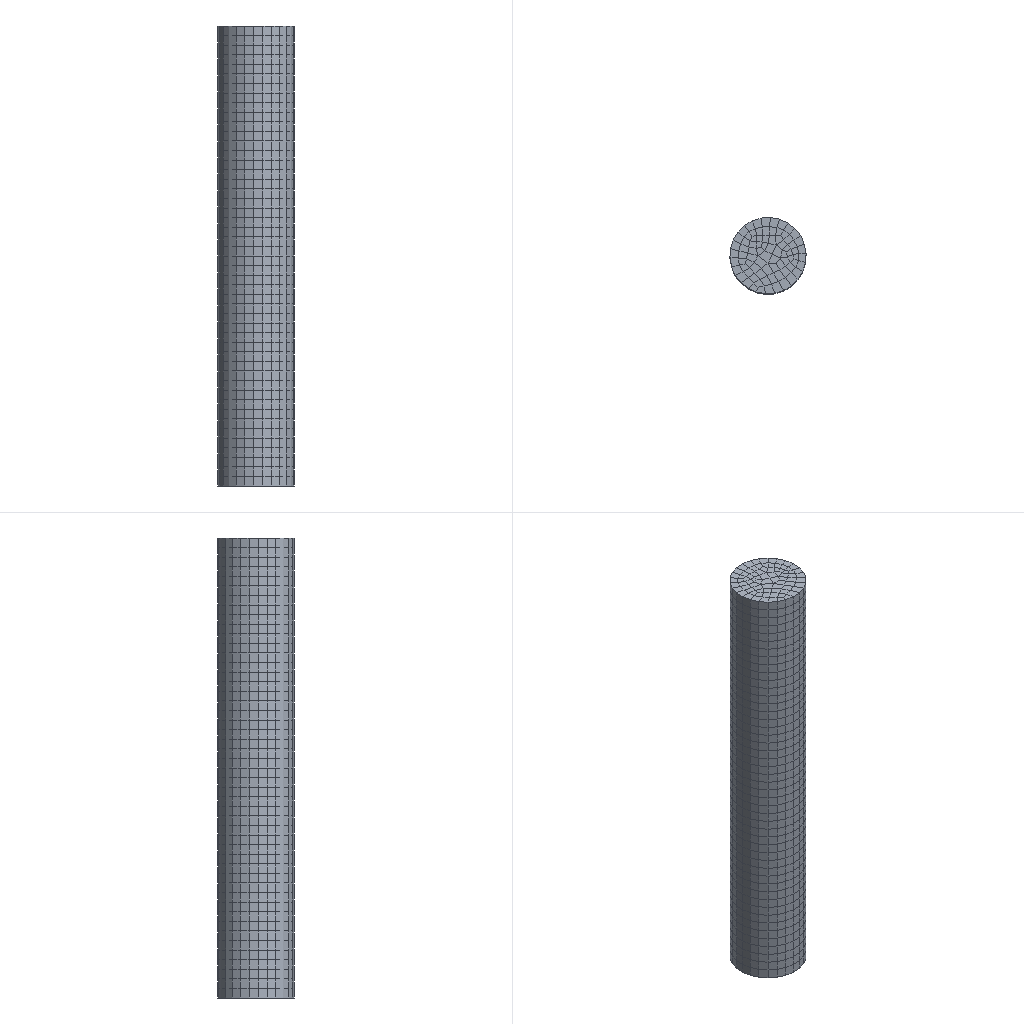Simulation study | abaqus
Set-up summary:
category,name,step,type,value,unit,region
solver,abaqus
solver,version,,,Abaqus/Explicit 2020
units,not stated in the deck,,not stated
analysis,deck,,transient,transient
load_step,Step-1,Step-1,transient
load_step,requested,,,1
mesh,nodes,,,17527
mesh,elements,,,16895
element_type,R3D3,,rigid,133
element_type,R3D4,,rigid,12970
element_type,C3D8R,,solid,3792
load,load commands in deck,,count,1
bc,support commands in deck,,count,7
material,TI,,in results
check,setup vs results,,match,"per instance, exact: element labels, types and connectivity; labels of the nodes the elements use; coordinates of those nodes at SINGLE_PRECISION in 3 of 3 instance(s)"
Abaqus input file, long lists of numbers shortened:
*Heading
** Job name: Job-2 Model name: Model-1-Copy
** Generated by: Abaqus/CAE 2020
*Preprint, echo=NO, model=NO, history=NO, contact=NO
**
** PARTS
**
*Part, name=chudun-2
*Node
      1,  -88.649,  -41.876,          90.
      2,  -88.649,  -41.876,         120.
** (8718 more lines like these left out)
*Element, type=R3D4
  1,    1,    7,  341,  388
  2,    7,    8,  342,  341
** (8690 more lines like these left out)
*Element, type=R3D3
6564, 7699, 6751, 7323
6565, 7752, 7314, 7227
** (54 more lines like these left out)
*Node
   8721,  -88.649,  -53.376,         120.
*Nset, nset=chudun-2-RefPt_, internal
8721,
*Elset, elset=chudun-2, generate
    1,  8748,     1
*End Part
**
*Part, name=chudun-4
*Node
      1,  -112.249,  -53.376,          26.
      2,  -112.249,  -53.376,          25.
** (4246 more lines like these left out)
*Element, type=R3D4
  1,   1,   6, 201,   2
  2,   6,   7, 200, 201
** (4276 more lines like these left out)
*Element, type=R3D3
1030, 1328, 1304, 1303
1031, 1332, 1323, 1294
** (75 more lines like these left out)
*Node
   4249,  -88.649,  -53.376,          26.
*Nset, nset=chudun-4-RefPt_, internal
4249,
*Elset, elset=chudun-4, generate
    1,  4355,     1
*End Part
**
*Part, name=xiancai
*Node
      1,   1.19,   3.819,   48.2
      2,  0.2415,   3.993,   48.2
** (4555 more lines like these left out)
*Element, type=C3D8R
   1,  109,   94,  133,  120,   16,    1,   40,   27
   2,  121,   95,  110,  134,   28,    2,   17,   41
** (3790 more lines like these left out)
*Nset, nset=Set-1, generate
    1,  4557,     1
*Elset, elset=Set-1, generate
    1,  3792,     1
** Section: Section-1
*Solid Section, elset=Set-1, material=ti
,
*End Part
**
**
** ASSEMBLY
**
*Assembly, name=Assembly
**
*Instance, name=xiancai-1, part=xiancai
          0.,           0.,        -104.
*End Instance
**
*Instance, name=chudun-2-1, part=chudun-2
   88.649,    53.376,        -120.
*End Instance
**
*Instance, name=chudun-4-1, part=chudun-4
   88.649,   -53.376,         -79.
   88.649,   -53.376,         -79.,    89.649,   -53.376,         -79.,         180.
*End Instance
**
*Nset, nset=Set-2, instance=xiancai-1, generate
 4465,  4557,     1
*Elset, elset=Set-2, instance=xiancai-1, generate
 3714,  3792,     1
*Nset, nset=Set-3, instance=chudun-2-1
 8721,
*Nset, nset=Set-3, instance=chudun-4-1
 4249,
*Nset, nset=Set-4, instance=xiancai-1, generate
  1,  93,   1
*Elset, elset=Set-4, instance=xiancai-1, generate
  1,  79,   1
*Nset, nset=Set-5, instance=chudun-2-1
 8721,
*Nset, nset=Set-5, instance=chudun-4-1
 4249,
*Rigid Body, ref node=chudun-2-1.chudun-2-RefPt_, elset=chudun-2-1.chudun-2
*Rigid Body, ref node=chudun-4-1.chudun-4-RefPt_, elset=chudun-4-1.chudun-4
*End Assembly
*Amplitude, name=Amp-1
             0.,              0.,             0.1,              1.
**
** MATERIALS
**
*Material, name=ti
*Density
 3.5e-09,
*Elastic
45000., 0.28
*Plastic
300.,0.
**
** INTERACTION PROPERTIES
**
*Surface Interaction, name=IntProp-1
*Friction
 0.01,
*Surface Behavior, pressure-overclosure=HARD
** ----------------------------------------------------------------
**
** STEP: Step-1
**
*Step, name=Step-1, nlgeom=YES
*Dynamic, Explicit
, 0.1
*Bulk Viscosity
0.06, 1.2
** Mass Scaling: Semi-Automatic
**               Whole Model
*Fixed Mass Scaling, factor=5000.
**
** BOUNDARY CONDITIONS
**
** Name: BC-1 Type: 对称/反对称/完全固定
*Boundary
Set-5, ENCASTRE
** Name: BC-2 Type: 位移/转角
*Boundary, amplitude=Amp-1
Set-4, 1, 1
Set-4, 2, 2
Set-4, 3, 3, -25.
Set-4, 4, 4
Set-4, 5, 5
Set-4, 6, 6
**
** INTERACTIONS
**
** Interaction: Int-1
*Contact, op=NEW
*Contact Inclusions, ALL EXTERIOR
*Contact Property Assignment
 ,  , IntProp-1
**
** OUTPUT REQUESTS
**
*Restart, write, number interval=1, time marks=NO
**
** FIELD OUTPUT: F-Output-1
**
*Output, field, number interval=50
*Node Output
A, RF, RM, RT, U, V
*Element Output, directions=YES
E, EVF, LE, MISES, PE, PEEQ, PEEQVAVG, PEVAVG, S, SVAVG
*Contact Output
CDISP, CSTRESS, PPRESS
**
** HISTORY OUTPUT: H-Output-1
**
*Output, history, variable=PRESELECT
*End Step
Results summary:
result,step,Step-1,completed,increments=29790 time=0.1/0.1
result,analysis,,,transient
result,last_loadstep,,,1
result,primary field,,,U
result,reaction total,,FX,154.575,model units
result,reaction total,,FY,478.181,model units
result,reaction total,,FZ,233.678,model units